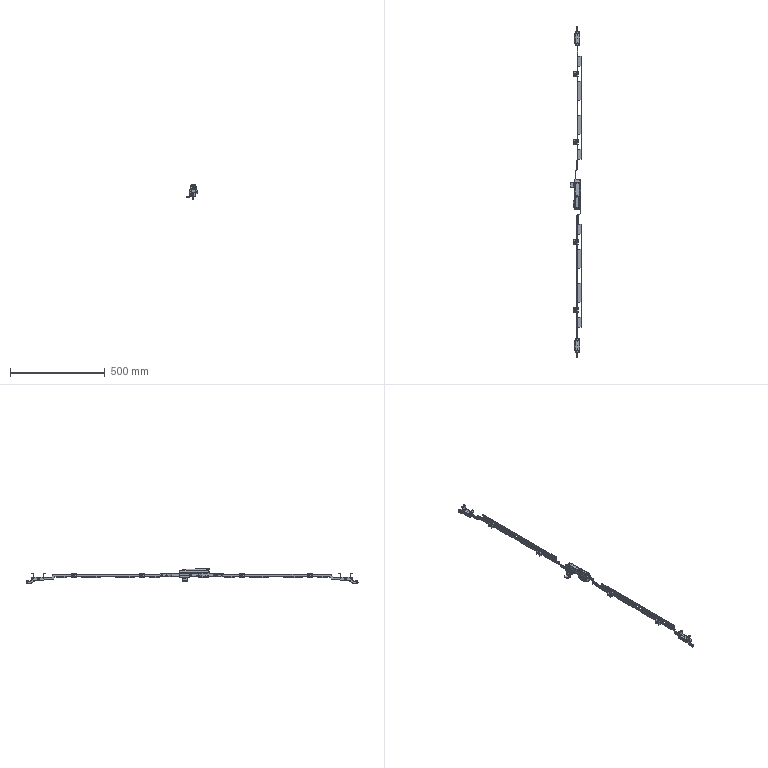Part | SolidWorks | 15 solids | 3848 faces | volume 356817 mm3 | plane 2013 | cylinder 1179 | spline 567 | cone 74 | torus 15 | commonest cylinder face diameters 1 x235 4.1 x102 2 x89 4.8 x86 3 x63 0.2 x61